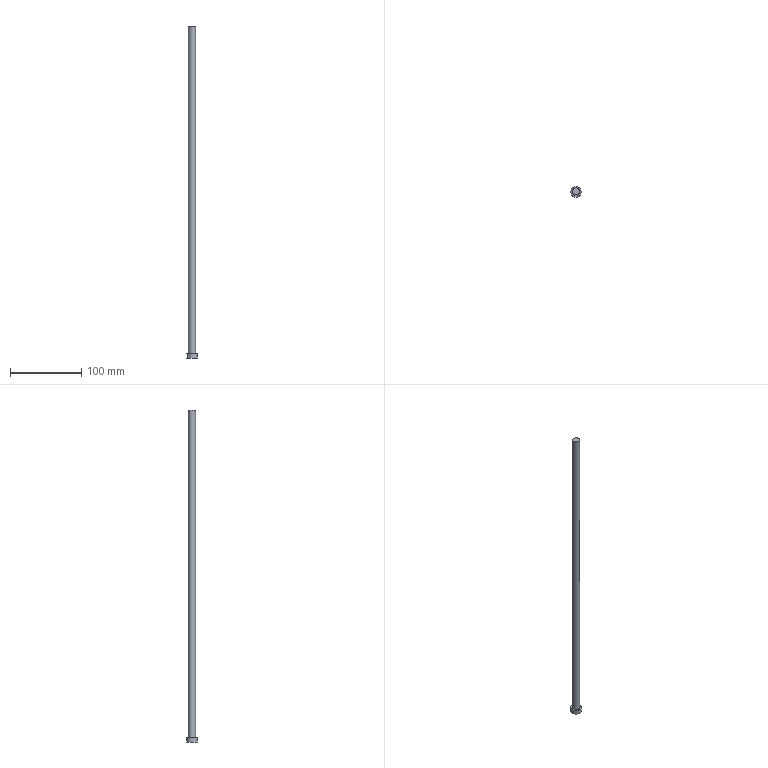Part | STEP file | solid 70 | 1 solid | 5 faces | box 15 x 15 x 466.378 mm | volume 37218 mm3 | plane 3 | cylinder 2 | commonest cylinder face diameters 10 x1 15 x1